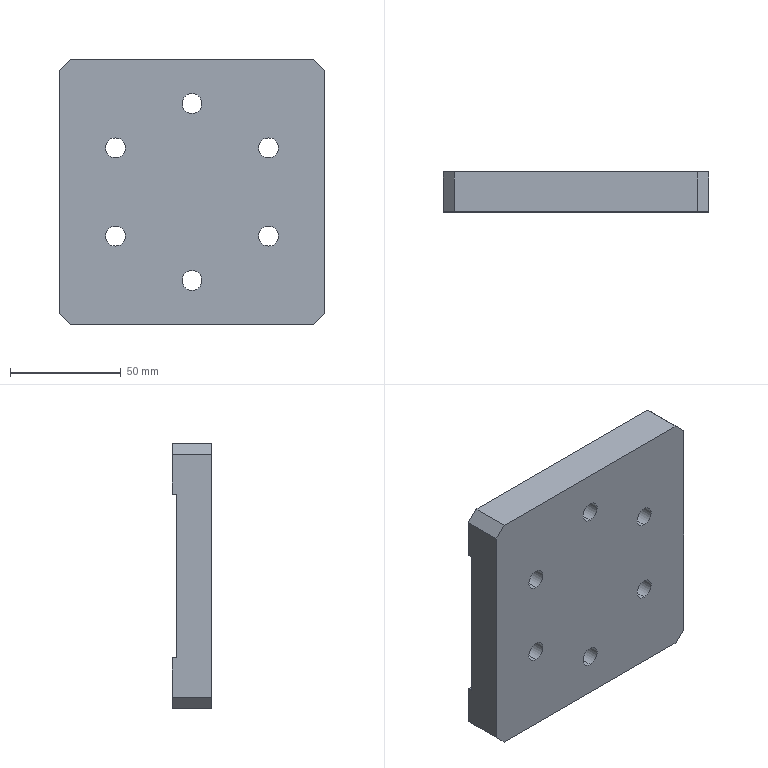Part | 1 solid | 46 faces | box 120 x 18 x 120 mm | volume 228068 mm3 | cylinder 24 | plane 22 | commonest cylinder face diameters 9 x12 15 x12
STEP:
#1=CARTESIAN_POINT('',(0.,7.4,-47.5));
#2=VERTEX_POINT('',#1);
#3=CARTESIAN_POINT('',(0.,7.4,-32.5));
#4=VERTEX_POINT('',#3);
#5=CARTESIAN_POINT('',(0.,7.4,-40.));
#6=DIRECTION('',(0.,1.,0.));
#7=DIRECTION('',(0.,0.,1.));
#8=AXIS2_PLACEMENT_3D('',#5,#6,#7);
#9=CIRCLE('',#8,7.5);
#10=EDGE_CURVE('',#2,#4,#9,.T.);
#11=ORIENTED_EDGE('',*,*,#10,.F.);
#12=CARTESIAN_POINT('',(0.,18.,-47.5));
#13=VERTEX_POINT('',#12);
#14=CARTESIAN_POINT('',(0.,18.,-47.5));
#15=DIRECTION('',(0.,1.,0.));
#16=VECTOR('',#15,1000.);
#17=LINE('',#14,#16);
#18=EDGE_CURVE('',#2,#13,#17,.T.);
#19=ORIENTED_EDGE('',*,*,#18,.T.);
#20=CARTESIAN_POINT('',(-6.874,18.,-37.));
#21=VERTEX_POINT('',#20);
#22=CARTESIAN_POINT('',(0.,18.,-40.));
#23=DIRECTION('',(0.,1.,0.));
#24=DIRECTION('',(0.,0.,1.));
#25=AXIS2_PLACEMENT_3D('',#22,#23,#24);
#26=CIRCLE('',#25,7.5);
#27=EDGE_CURVE('',#13,#21,#26,.T.);
#28=ORIENTED_EDGE('',*,*,#27,.T.);
#29=CARTESIAN_POINT('',(-6.874,16.,-37.));
#30=VERTEX_POINT('',#29);
#31=CARTESIAN_POINT('',(-6.874,18.,-37.));
#32=DIRECTION('',(0.,-1.,0.));
#33=VECTOR('',#32,1000.);
#34=LINE('',#31,#33);
#35=EDGE_CURVE('',#21,#30,#34,.T.);
#36=ORIENTED_EDGE('',*,*,#35,.T.);
#37=CARTESIAN_POINT('',(0.,16.,-32.5));
#38=VERTEX_POINT('',#37);
#39=CARTESIAN_POINT('',(0.,16.,-40.));
#40=DIRECTION('',(0.,1.,0.));
#41=DIRECTION('',(0.,0.,-1.));
#42=AXIS2_PLACEMENT_3D('',#39,#40,#41);
#43=CIRCLE('',#42,7.5);
#44=EDGE_CURVE('',#30,#38,#43,.T.);
#45=ORIENTED_EDGE('',*,*,#44,.T.);
#46=CARTESIAN_POINT('',(0.,18.,-32.5));
#47=DIRECTION('',(0.,1.,0.));
#48=VECTOR('',#47,1000.);
#49=LINE('',#46,#48);
#50=EDGE_CURVE('',#4,#38,#49,.T.);
#51=ORIENTED_EDGE('',*,*,#50,.F.);
#52=EDGE_LOOP('',(#11,#19,#28,#36,#45,#51));
#53=FACE_OUTER_BOUND('',#52,.T.);
#54=CARTESIAN_POINT('',(0.,18.,-40.));
#55=DIRECTION('',(0.,1.,0.));
#56=DIRECTION('',(0.,0.,1.));
#57=AXIS2_PLACEMENT_3D('',#54,#55,#56);
#58=CYLINDRICAL_SURFACE('',#57,7.5);
#59=ADVANCED_FACE('',(#53),#58,.F.);
#60=CARTESIAN_POINT('',(0.,0.,-44.5));
#61=VERTEX_POINT('',#60);
#62=CARTESIAN_POINT('',(0.,0.,-35.5));
#63=VERTEX_POINT('',#62);
#64=CARTESIAN_POINT('',(0.,0.,-40.));
#65=DIRECTION('',(0.,1.,0.));
#66=DIRECTION('',(0.,0.,1.));
#67=AXIS2_PLACEMENT_3D('',#64,#65,#66);
#68=CIRCLE('',#67,4.5);
#69=EDGE_CURVE('',#61,#63,#68,.T.);
#70=ORIENTED_EDGE('',*,*,#69,.F.);
#71=CARTESIAN_POINT('',(0.,7.4,-44.5));
#72=VERTEX_POINT('',#71);
#73=CARTESIAN_POINT('',(0.,18.,-44.5));
#74=DIRECTION('',(0.,1.,0.));
#75=VECTOR('',#74,1000.);
#76=LINE('',#73,#75);
#77=EDGE_CURVE('',#61,#72,#76,.T.);
#78=ORIENTED_EDGE('',*,*,#77,.T.);
#79=CARTESIAN_POINT('',(0.,7.4,-35.5));
#80=VERTEX_POINT('',#79);
#81=CARTESIAN_POINT('',(0.,7.4,-40.));
#82=DIRECTION('',(0.,1.,0.));
#83=DIRECTION('',(0.,0.,1.));
#84=AXIS2_PLACEMENT_3D('',#81,#82,#83);
#85=CIRCLE('',#84,4.5);
#86=EDGE_CURVE('',#72,#80,#85,.T.);
#87=ORIENTED_EDGE('',*,*,#86,.T.);
#88=CARTESIAN_POINT('',(0.,18.,-35.5));
#89=DIRECTION('',(0.,1.,0.));
#90=VECTOR('',#89,1000.);
#91=LINE('',#88,#90);
#92=EDGE_CURVE('',#63,#80,#91,.T.);
#93=ORIENTED_EDGE('',*,*,#92,.F.);
#94=EDGE_LOOP('',(#70,#78,#87,#93));
#95=FACE_OUTER_BOUND('',#94,.T.);
#96=CARTESIAN_POINT('',(0.,18.,-40.));
#97=DIRECTION('',(0.,1.,0.));
#98=DIRECTION('',(0.,0.,1.));
#99=AXIS2_PLACEMENT_3D('',#96,#97,#98);
#100=CYLINDRICAL_SURFACE('',#99,4.5);
#101=ADVANCED_FACE('',(#95),#100,.F.);
#102=CARTESIAN_POINT('',(-34.641,7.4,-27.5));
#103=VERTEX_POINT('',#102);
#104=CARTESIAN_POINT('',(-34.641,7.4,-12.5));
#105=VERTEX_POINT('',#104);
#106=CARTESIAN_POINT('',(-34.641,7.4,-20.));
#107=DIRECTION('',(0.,1.,0.));
#108=DIRECTION('',(0.,0.,1.));
#109=AXIS2_PLACEMENT_3D('',#106,#107,#108);
#110=CIRCLE('',#109,7.5);
#111=EDGE_CURVE('',#103,#105,#110,.T.);
#112=ORIENTED_EDGE('',*,*,#111,.F.);
#113=CARTESIAN_POINT('',(-34.641,16.,-27.5));
#114=VERTEX_POINT('',#113);
#115=CARTESIAN_POINT('',(-34.641,18.,-27.5));
#116=DIRECTION('',(0.,1.,0.));
#117=VECTOR('',#116,1000.);
#118=LINE('',#115,#117);
#119=EDGE_CURVE('',#103,#114,#118,.T.);
#120=ORIENTED_EDGE('',*,*,#119,.T.);
#121=CARTESIAN_POINT('',(-34.641,16.,-12.5));
#122=VERTEX_POINT('',#121);
#123=CARTESIAN_POINT('',(-34.641,16.,-20.));
#124=DIRECTION('',(0.,1.,0.));
#125=DIRECTION('',(0.,0.,-1.));
#126=AXIS2_PLACEMENT_3D('',#123,#124,#125);
#127=CIRCLE('',#126,7.5);
#128=EDGE_CURVE('',#114,#122,#127,.T.);
#129=ORIENTED_EDGE('',*,*,#128,.T.);
#130=CARTESIAN_POINT('',(-34.641,18.,-12.5));
#131=DIRECTION('',(0.,1.,0.));
#132=VECTOR('',#131,1000.);
#133=LINE('',#130,#132);
#134=EDGE_CURVE('',#105,#122,#133,.T.);
#135=ORIENTED_EDGE('',*,*,#134,.F.);
#136=EDGE_LOOP('',(#112,#120,#129,#135));
#137=FACE_OUTER_BOUND('',#136,.T.);
#138=CARTESIAN_POINT('',(-34.641,18.,-20.));
#139=DIRECTION('',(0.,1.,0.));
#140=DIRECTION('',(0.,0.,1.));
#141=AXIS2_PLACEMENT_3D('',#138,#139,#140);
#142=CYLINDRICAL_SURFACE('',#141,7.5);
#143=ADVANCED_FACE('',(#137),#142,.F.);
#144=CARTESIAN_POINT('',(-34.641,0.,-24.5));
#145=VERTEX_POINT('',#144);
#146=CARTESIAN_POINT('',(-34.641,0.,-15.5));
#147=VERTEX_POINT('',#146);
#148=CARTESIAN_POINT('',(-34.641,0.,-20.));
#149=DIRECTION('',(0.,1.,0.));
#150=DIRECTION('',(0.,0.,1.));
#151=AXIS2_PLACEMENT_3D('',#148,#149,#150);
#152=CIRCLE('',#151,4.5);
#153=EDGE_CURVE('',#145,#147,#152,.T.);
#154=ORIENTED_EDGE('',*,*,#153,.F.);
#155=CARTESIAN_POINT('',(-34.641,7.4,-24.5));
#156=VERTEX_POINT('',#155);
#157=CARTESIAN_POINT('',(-34.641,18.,-24.5));
#158=DIRECTION('',(0.,1.,0.));
#159=VECTOR('',#158,1000.);
#160=LINE('',#157,#159);
#161=EDGE_CURVE('',#145,#156,#160,.T.);
#162=ORIENTED_EDGE('',*,*,#161,.T.);
#163=CARTESIAN_POINT('',(-34.641,7.4,-15.5));
#164=VERTEX_POINT('',#163);
#165=CARTESIAN_POINT('',(-34.641,7.4,-20.));
#166=DIRECTION('',(0.,1.,0.));
#167=DIRECTION('',(0.,0.,1.));
#168=AXIS2_PLACEMENT_3D('',#165,#166,#167);
#169=CIRCLE('',#168,4.5);
#170=EDGE_CURVE('',#156,#164,#169,.T.);
#171=ORIENTED_EDGE('',*,*,#170,.T.);
#172=CARTESIAN_POINT('',(-34.641,18.,-15.5));
#173=DIRECTION('',(0.,1.,0.));
#174=VECTOR('',#173,1000.);
#175=LINE('',#172,#174);
#176=EDGE_CURVE('',#147,#164,#175,.T.);
#177=ORIENTED_EDGE('',*,*,#176,.F.);
#178=EDGE_LOOP('',(#154,#162,#171,#177));
#179=FACE_OUTER_BOUND('',#178,.T.);
#180=CARTESIAN_POINT('',(-34.641,18.,-20.));
#181=DIRECTION('',(0.,1.,0.));
#182=DIRECTION('',(0.,0.,1.));
#183=AXIS2_PLACEMENT_3D('',#180,#181,#182);
#184=CYLINDRICAL_SURFACE('',#183,4.5);
#185=ADVANCED_FACE('',(#179),#184,.F.);
#186=CARTESIAN_POINT('',(-34.641,7.4,12.5));
#187=VERTEX_POINT('',#186);
#188=CARTESIAN_POINT('',(-34.641,7.4,27.5));
#189=VERTEX_POINT('',#188);
#190=CARTESIAN_POINT('',(-34.641,7.4,20.));
#191=DIRECTION('',(0.,1.,0.));
#192=DIRECTION('',(0.,0.,1.));
#193=AXIS2_PLACEMENT_3D('',#190,#191,#192);
#194=CIRCLE('',#193,7.5);
#195=EDGE_CURVE('',#187,#189,#194,.T.);
#196=ORIENTED_EDGE('',*,*,#195,.F.);
#197=CARTESIAN_POINT('',(-34.641,16.,12.5));
#198=VERTEX_POINT('',#197);
#199=CARTESIAN_POINT('',(-34.641,18.,12.5));
#200=DIRECTION('',(0.,1.,0.));
#201=VECTOR('',#200,1000.);
#202=LINE('',#199,#201);
#203=EDGE_CURVE('',#187,#198,#202,.T.);
#204=ORIENTED_EDGE('',*,*,#203,.T.);
#205=CARTESIAN_POINT('',(-34.641,16.,27.5));
#206=VERTEX_POINT('',#205);
#207=CARTESIAN_POINT('',(-34.641,16.,20.));
#208=DIRECTION('',(0.,1.,0.));
#209=DIRECTION('',(0.,0.,-1.));
#210=AXIS2_PLACEMENT_3D('',#207,#208,#209);
#211=CIRCLE('',#210,7.5);
#212=EDGE_CURVE('',#198,#206,#211,.T.);
#213=ORIENTED_EDGE('',*,*,#212,.T.);
#214=CARTESIAN_POINT('',(-34.641,18.,27.5));
#215=DIRECTION('',(0.,1.,0.));
#216=VECTOR('',#215,1000.);
#217=LINE('',#214,#216);
#218=EDGE_CURVE('',#189,#206,#217,.T.);
#219=ORIENTED_EDGE('',*,*,#218,.F.);
#220=EDGE_LOOP('',(#196,#204,#213,#219));
#221=FACE_OUTER_BOUND('',#220,.T.);
#222=CARTESIAN_POINT('',(-34.641,18.,20.));
#223=DIRECTION('',(0.,1.,0.));
#224=DIRECTION('',(0.,0.,1.));
#225=AXIS2_PLACEMENT_3D('',#222,#223,#224);
#226=CYLINDRICAL_SURFACE('',#225,7.5);
#227=ADVANCED_FACE('',(#221),#226,.F.);
#228=CARTESIAN_POINT('',(-34.641,0.,15.5));
#229=VERTEX_POINT('',#228);
#230=CARTESIAN_POINT('',(-34.641,0.,24.5));
#231=VERTEX_POINT('',#230);
#232=CARTESIAN_POINT('',(-34.641,0.,20.));
#233=DIRECTION('',(0.,1.,0.));
#234=DIRECTION('',(0.,0.,1.));
#235=AXIS2_PLACEMENT_3D('',#232,#233,#234);
#236=CIRCLE('',#235,4.5);
#237=EDGE_CURVE('',#229,#231,#236,.T.);
#238=ORIENTED_EDGE('',*,*,#237,.F.);
#239=CARTESIAN_POINT('',(-34.641,7.4,15.5));
#240=VERTEX_POINT('',#239);
#241=CARTESIAN_POINT('',(-34.641,18.,15.5));
#242=DIRECTION('',(0.,1.,0.));
#243=VECTOR('',#242,1000.);
#244=LINE('',#241,#243);
#245=EDGE_CURVE('',#229,#240,#244,.T.);
#246=ORIENTED_EDGE('',*,*,#245,.T.);
#247=CARTESIAN_POINT('',(-34.641,7.4,24.5));
#248=VERTEX_POINT('',#247);
#249=CARTESIAN_POINT('',(-34.641,7.4,20.));
#250=DIRECTION('',(0.,1.,0.));
#251=DIRECTION('',(0.,0.,1.));
#252=AXIS2_PLACEMENT_3D('',#249,#250,#251);
#253=CIRCLE('',#252,4.5);
#254=EDGE_CURVE('',#240,#248,#253,.T.);
#255=ORIENTED_EDGE('',*,*,#254,.T.);
#256=CARTESIAN_POINT('',(-34.641,18.,24.5));
#257=DIRECTION('',(0.,1.,0.));
#258=VECTOR('',#257,1000.);
#259=LINE('',#256,#258);
#260=EDGE_CURVE('',#231,#248,#259,.T.);
#261=ORIENTED_EDGE('',*,*,#260,.F.);
#262=EDGE_LOOP('',(#238,#246,#255,#261));
#263=FACE_OUTER_BOUND('',#262,.T.);
#264=CARTESIAN_POINT('',(-34.641,18.,20.));
#265=DIRECTION('',(0.,1.,0.));
#266=DIRECTION('',(0.,0.,1.));
#267=AXIS2_PLACEMENT_3D('',#264,#265,#266);
#268=CYLINDRICAL_SURFACE('',#267,4.5);
#269=ADVANCED_FACE('',(#263),#268,.F.);
#270=CARTESIAN_POINT('',(0.,7.4,32.5));
#271=VERTEX_POINT('',#270);
#272=CARTESIAN_POINT('',(0.,7.4,47.5));
#273=VERTEX_POINT('',#272);
#274=CARTESIAN_POINT('',(0.,7.4,40.));
#275=DIRECTION('',(0.,1.,0.));
#276=DIRECTION('',(0.,0.,1.));
#277=AXIS2_PLACEMENT_3D('',#274,#275,#276);
#278=CIRCLE('',#277,7.5);
#279=EDGE_CURVE('',#271,#273,#278,.T.);
#280=ORIENTED_EDGE('',*,*,#279,.F.);
#281=CARTESIAN_POINT('',(0.,16.,32.5));
#282=VERTEX_POINT('',#281);
#283=CARTESIAN_POINT('',(0.,18.,32.5));
#284=DIRECTION('',(0.,1.,0.));
#285=VECTOR('',#284,1000.);
#286=LINE('',#283,#285);
#287=EDGE_CURVE('',#271,#282,#286,.T.);
#288=ORIENTED_EDGE('',*,*,#287,.T.);
#289=CARTESIAN_POINT('',(-6.874,16.,37.));
#290=VERTEX_POINT('',#289);
#291=CARTESIAN_POINT('',(0.,16.,40.));
#292=DIRECTION('',(0.,1.,0.));
#293=DIRECTION('',(0.,0.,-1.));
#294=AXIS2_PLACEMENT_3D('',#291,#292,#293);
#295=CIRCLE('',#294,7.5);
#296=EDGE_CURVE('',#282,#290,#295,.T.);
#297=ORIENTED_EDGE('',*,*,#296,.T.);
#298=CARTESIAN_POINT('',(-6.874,18.,37.));
#299=VERTEX_POINT('',#298);
#300=CARTESIAN_POINT('',(-6.874,18.,37.));
#301=DIRECTION('',(0.,1.,0.));
#302=VECTOR('',#301,1000.);
#303=LINE('',#300,#302);
#304=EDGE_CURVE('',#290,#299,#303,.T.);
#305=ORIENTED_EDGE('',*,*,#304,.T.);
#306=CARTESIAN_POINT('',(0.,18.,47.5));
#307=VERTEX_POINT('',#306);
#308=CARTESIAN_POINT('',(0.,18.,40.));
#309=DIRECTION('',(0.,1.,0.));
#310=DIRECTION('',(0.,0.,1.));
#311=AXIS2_PLACEMENT_3D('',#308,#309,#310);
#312=CIRCLE('',#311,7.5);
#313=EDGE_CURVE('',#299,#307,#312,.T.);
#314=ORIENTED_EDGE('',*,*,#313,.T.);
#315=CARTESIAN_POINT('',(0.,18.,47.5));
#316=DIRECTION('',(0.,1.,0.));
#317=VECTOR('',#316,1000.);
#318=LINE('',#315,#317);
#319=EDGE_CURVE('',#273,#307,#318,.T.);
#320=ORIENTED_EDGE('',*,*,#319,.F.);
#321=EDGE_LOOP('',(#280,#288,#297,#305,#314,#320));
#322=FACE_OUTER_BOUND('',#321,.T.);
#323=CARTESIAN_POINT('',(0.,18.,40.));
#324=DIRECTION('',(0.,1.,0.));
#325=DIRECTION('',(0.,0.,1.));
#326=AXIS2_PLACEMENT_3D('',#323,#324,#325);
#327=CYLINDRICAL_SURFACE('',#326,7.5);
#328=ADVANCED_FACE('',(#322),#327,.F.);
#329=CARTESIAN_POINT('',(0.,0.,35.5));
#330=VERTEX_POINT('',#329);
#331=CARTESIAN_POINT('',(0.,0.,44.5));
#332=VERTEX_POINT('',#331);
#333=CARTESIAN_POINT('',(0.,0.,40.));
#334=DIRECTION('',(0.,1.,0.));
#335=DIRECTION('',(0.,0.,1.));
#336=AXIS2_PLACEMENT_3D('',#333,#334,#335);
#337=CIRCLE('',#336,4.5);
#338=EDGE_CURVE('',#330,#332,#337,.T.);
#339=ORIENTED_EDGE('',*,*,#338,.F.);
#340=CARTESIAN_POINT('',(0.,7.4,35.5));
#341=VERTEX_POINT('',#340);
#342=CARTESIAN_POINT('',(0.,18.,35.5));
#343=DIRECTION('',(0.,1.,0.));
#344=VECTOR('',#343,1000.);
#345=LINE('',#342,#344);
#346=EDGE_CURVE('',#330,#341,#345,.T.);
#347=ORIENTED_EDGE('',*,*,#346,.T.);
#348=CARTESIAN_POINT('',(0.,7.4,44.5));
#349=VERTEX_POINT('',#348);
#350=CARTESIAN_POINT('',(0.,7.4,40.));
#351=DIRECTION('',(0.,1.,0.));
#352=DIRECTION('',(0.,0.,1.));
#353=AXIS2_PLACEMENT_3D('',#350,#351,#352);
#354=CIRCLE('',#353,4.5);
#355=EDGE_CURVE('',#341,#349,#354,.T.);
#356=ORIENTED_EDGE('',*,*,#355,.T.);
#357=CARTESIAN_POINT('',(0.,18.,44.5));
#358=DIRECTION('',(0.,1.,0.));
#359=VECTOR('',#358,1000.);
#360=LINE('',#357,#359);
#361=EDGE_CURVE('',#332,#349,#360,.T.);
#362=ORIENTED_EDGE('',*,*,#361,.F.);
#363=EDGE_LOOP('',(#339,#347,#356,#362));
#364=FACE_OUTER_BOUND('',#363,.T.);
#365=CARTESIAN_POINT('',(0.,18.,40.));
#366=DIRECTION('',(0.,1.,0.));
#367=DIRECTION('',(0.,0.,1.));
#368=AXIS2_PLACEMENT_3D('',#365,#366,#367);
#369=CYLINDRICAL_SURFACE('',#368,4.5);
#370=ADVANCED_FACE('',(#364),#369,.F.);
#371=CARTESIAN_POINT('',(34.641,7.4,12.5));
#372=VERTEX_POINT('',#371);
#373=CARTESIAN_POINT('',(34.641,7.4,27.5));
#374=VERTEX_POINT('',#373);
#375=CARTESIAN_POINT('',(34.641,7.4,20.));
#376=DIRECTION('',(0.,1.,0.));
#377=DIRECTION('',(0.,0.,1.));
#378=AXIS2_PLACEMENT_3D('',#375,#376,#377);
#379=CIRCLE('',#378,7.5);
#380=EDGE_CURVE('',#372,#374,#379,.T.);
#381=ORIENTED_EDGE('',*,*,#380,.F.);
#382=CARTESIAN_POINT('',(34.641,16.,12.5));
#383=VERTEX_POINT('',#382);
#384=CARTESIAN_POINT('',(34.641,18.,12.5));
#385=DIRECTION('',(0.,1.,0.));
#386=VECTOR('',#385,1000.);
#387=LINE('',#384,#386);
#388=EDGE_CURVE('',#372,#383,#387,.T.);
#389=ORIENTED_EDGE('',*,*,#388,.T.);
#390=CARTESIAN_POINT('',(34.641,16.,27.5));
#391=VERTEX_POINT('',#390);
#392=CARTESIAN_POINT('',(34.641,16.,20.));
#393=DIRECTION('',(0.,1.,0.));
#394=DIRECTION('',(0.,0.,-1.));
#395=AXIS2_PLACEMENT_3D('',#392,#393,#394);
#396=CIRCLE('',#395,7.5);
#397=EDGE_CURVE('',#383,#391,#396,.T.);
#398=ORIENTED_EDGE('',*,*,#397,.T.);
#399=CARTESIAN_POINT('',(34.641,18.,27.5));
#400=DIRECTION('',(0.,1.,0.));
#401=VECTOR('',#400,1000.);
#402=LINE('',#399,#401);
#403=EDGE_CURVE('',#374,#391,#402,.T.);
#404=ORIENTED_EDGE('',*,*,#403,.F.);
#405=EDGE_LOOP('',(#381,#389,#398,#404));
#406=FACE_OUTER_BOUND('',#405,.T.);
#407=CARTESIAN_POINT('',(34.641,18.,20.));
#408=DIRECTION('',(0.,1.,0.));
#409=DIRECTION('',(0.,0.,1.));
#410=AXIS2_PLACEMENT_3D('',#407,#408,#409);
#411=CYLINDRICAL_SURFACE('',#410,7.5);
#412=ADVANCED_FACE('',(#406),#411,.F.);
#413=CARTESIAN_POINT('',(34.641,0.,15.5));
#414=VERTEX_POINT('',#413);
#415=CARTESIAN_POINT('',(34.641,0.,24.5));
#416=VERTEX_POINT('',#415);
#417=CARTESIAN_POINT('',(34.641,0.,20.));
#418=DIRECTION('',(0.,1.,0.));
#419=DIRECTION('',(0.,0.,1.));
#420=AXIS2_PLACEMENT_3D('',#417,#418,#419);
#421=CIRCLE('',#420,4.5);
#422=EDGE_CURVE('',#414,#416,#421,.T.);
#423=ORIENTED_EDGE('',*,*,#422,.F.);
#424=CARTESIAN_POINT('',(34.641,7.4,15.5));
#425=VERTEX_POINT('',#424);
#426=CARTESIAN_POINT('',(34.641,18.,15.5));
#427=DIRECTION('',(0.,1.,0.));
#428=VECTOR('',#427,1000.);
#429=LINE('',#426,#428);
#430=EDGE_CURVE('',#414,#425,#429,.T.);
#431=ORIENTED_EDGE('',*,*,#430,.T.);
#432=CARTESIAN_POINT('',(34.641,7.4,24.5));
#433=VERTEX_POINT('',#432);
#434=CARTESIAN_POINT('',(34.641,7.4,20.));
#435=DIRECTION('',(0.,1.,0.));
#436=DIRECTION('',(0.,0.,1.));
#437=AXIS2_PLACEMENT_3D('',#434,#435,#436);
#438=CIRCLE('',#437,4.5);
#439=EDGE_CURVE('',#425,#433,#438,.T.);
#440=ORIENTED_EDGE('',*,*,#439,.T.);
#441=CARTESIAN_POINT('',(34.641,18.,24.5));
#442=DIRECTION('',(0.,1.,0.));
#443=VECTOR('',#442,1000.);
#444=LINE('',#441,#443);
#445=EDGE_CURVE('',#416,#433,#444,.T.);
#446=ORIENTED_EDGE('',*,*,#445,.F.);
#447=EDGE_LOOP('',(#423,#431,#440,#446));
#448=FACE_OUTER_BOUND('',#447,.T.);
#449=CARTESIAN_POINT('',(34.641,18.,20.));
#450=DIRECTION('',(0.,1.,0.));
#451=DIRECTION('',(0.,0.,1.));
#452=AXIS2_PLACEMENT_3D('',#449,#450,#451);
#453=CYLINDRICAL_SURFACE('',#452,4.5);
#454=ADVANCED_FACE('',(#448),#453,.F.);
#455=CARTESIAN_POINT('',(34.641,7.4,-27.5));
#456=VERTEX_POINT('',#455);
#457=CARTESIAN_POINT('',(34.641,7.4,-12.5));
#458=VERTEX_POINT('',#457);
#459=CARTESIAN_POINT('',(34.641,7.4,-20.));
#460=DIRECTION('',(0.,1.,0.));
#461=DIRECTION('',(0.,0.,1.));
#462=AXIS2_PLACEMENT_3D('',#459,#460,#461);
#463=CIRCLE('',#462,7.5);
#464=EDGE_CURVE('',#456,#458,#463,.T.);
#465=ORIENTED_EDGE('',*,*,#464,.F.);
#466=CARTESIAN_POINT('',(34.641,16.,-27.5));
#467=VERTEX_POINT('',#466);
#468=CARTESIAN_POINT('',(34.641,18.,-27.5));
#469=DIRECTION('',(0.,1.,0.));
#470=VECTOR('',#469,1000.);
#471=LINE('',#468,#470);
#472=EDGE_CURVE('',#456,#467,#471,.T.);
#473=ORIENTED_EDGE('',*,*,#472,.T.);
#474=CARTESIAN_POINT('',(34.641,16.,-12.5));
#475=VERTEX_POINT('',#474);
#476=CARTESIAN_POINT('',(34.641,16.,-20.));
#477=DIRECTION('',(0.,1.,0.));
#478=DIRECTION('',(0.,0.,-1.));
#479=AXIS2_PLACEMENT_3D('',#476,#477,#478);
#480=CIRCLE('',#479,7.5);
#481=EDGE_CURVE('',#467,#475,#480,.T.);
#482=ORIENTED_EDGE('',*,*,#481,.T.);
#483=CARTESIAN_POINT('',(34.641,18.,-12.5));
#484=DIRECTION('',(0.,1.,0.));
#485=VECTOR('',#484,1000.);
#486=LINE('',#483,#485);
#487=EDGE_CURVE('',#458,#475,#486,.T.);
#488=ORIENTED_EDGE('',*,*,#487,.F.);
#489=EDGE_LOOP('',(#465,#473,#482,#488));
#490=FACE_OUTER_BOUND('',#489,.T.);
#491=CARTESIAN_POINT('',(34.641,18.,-20.));
#492=DIRECTION('',(0.,1.,0.));
#493=DIRECTION('',(0.,0.,1.));
#494=AXIS2_PLACEMENT_3D('',#491,#492,#493);
#495=CYLINDRICAL_SURFACE('',#494,7.5);
#496=ADVANCED_FACE('',(#490),#495,.F.);
#497=CARTESIAN_POINT('',(34.641,0.,-24.5));
#498=VERTEX_POINT('',#497);
#499=CARTESIAN_POINT('',(34.641,0.,-15.5));
#500=VERTEX_POINT('',#499);
#501=CARTESIAN_POINT('',(34.641,0.,-20.));
#502=DIRECTION('',(0.,1.,0.));
#503=DIRECTION('',(0.,0.,1.));
#504=AXIS2_PLACEMENT_3D('',#501,#502,#503);
#505=CIRCLE('',#504,4.5);
#506=EDGE_CURVE('',#498,#500,#505,.T.);
#507=ORIENTED_EDGE('',*,*,#506,.F.);
#508=CARTESIAN_POINT('',(34.641,7.4,-24.5));
#509=VERTEX_POINT('',#508);
#510=CARTESIAN_POINT('',(34.641,18.,-24.5));
#511=DIRECTION('',(0.,1.,0.));
#512=VECTOR('',#511,1000.);
#513=LINE('',#510,#512);
#514=EDGE_CURVE('',#498,#509,#513,.T.);
#515=ORIENTED_EDGE('',*,*,#514,.T.);
#516=CARTESIAN_POINT('',(34.641,7.4,-15.5));
#517=VERTEX_POINT('',#516);
#518=CARTESIAN_POINT('',(34.641,7.4,-20.));
#519=DIRECTION('',(0.,1.,0.));
#520=DIRECTION('',(0.,0.,1.));
#521=AXIS2_PLACEMENT_3D('',#518,#519,#520);
#522=CIRCLE('',#521,4.5);
#523=EDGE_CURVE('',#509,#517,#522,.T.);
#524=ORIENTED_EDGE('',*,*,#523,.T.);
#525=CARTESIAN_POINT('',(34.641,18.,-15.5));
#526=DIRECTION('',(0.,1.,0.));
#527=VECTOR('',#526,1000.);
#528=LINE('',#525,#527);
#529=EDGE_CURVE('',#500,#517,#528,.T.);
#530=ORIENTED_EDGE('',*,*,#529,.F.);
#531=EDGE_LOOP('',(#507,#515,#524,#530));
#532=FACE_OUTER_BOUND('',#531,.T.);
#533=CARTESIAN_POINT('',(34.641,18.,-20.));
#534=DIRECTION('',(0.,1.,0.));
#535=DIRECTION('',(0.,0.,1.));
#536=AXIS2_PLACEMENT_3D('',#533,#534,#535);
#537=CYLINDRICAL_SURFACE('',#536,4.5);
#538=ADVANCED_FACE('',(#532),#537,.F.);
#539=CARTESIAN_POINT('',(-55.,18.,60.));
#540=VERTEX_POINT('',#539);
#541=CARTESIAN_POINT('',(55.,18.,60.));
#542=VERTEX_POINT('',#541);
#543=CARTESIAN_POINT('',(-60.,18.,60.));
#544=DIRECTION('',(1.,0.,0.));
#545=VECTOR('',#544,1000.);
#546=LINE('',#543,#545);
#547=EDGE_CURVE('',#540,#542,#546,.T.);
#548=ORIENTED_EDGE('',*,*,#547,.T.);
#549=CARTESIAN_POINT('',(60.,18.,55.));
#550=VERTEX_POINT('',#549);
#551=CARTESIAN_POINT('',(60.,18.,55.));
#552=DIRECTION('',(0.7071,0.,-0.7071));
#553=VECTOR('',#552,1000.);
#554=LINE('',#551,#553);
#555=EDGE_CURVE('',#542,#550,#554,.T.);
#556=ORIENTED_EDGE('',*,*,#555,.T.);
#557=CARTESIAN_POINT('',(60.,18.,37.));
#558=VERTEX_POINT('',#557);
#559=CARTESIAN_POINT('',(60.,18.,60.));
#560=DIRECTION('',(0.,0.,-1.));
#561=VECTOR('',#560,1000.);
#562=LINE('',#559,#561);
#563=EDGE_CURVE('',#550,#558,#562,.T.);
#564=ORIENTED_EDGE('',*,*,#563,.T.);
#565=CARTESIAN_POINT('',(6.874,18.,37.));
#566=VERTEX_POINT('',#565);
#567=CARTESIAN_POINT('',(-60.,18.,37.));
#568=DIRECTION('',(1.,0.,0.));
#569=VECTOR('',#568,1000.);
#570=LINE('',#567,#569);
#571=EDGE_CURVE('',#566,#558,#570,.T.);
#572=ORIENTED_EDGE('',*,*,#571,.F.);
#573=CARTESIAN_POINT('',(0.,18.,40.));
#574=DIRECTION('',(0.,1.,0.));
#575=DIRECTION('',(0.,0.,1.));
#576=AXIS2_PLACEMENT_3D('',#573,#574,#575);
#577=CIRCLE('',#576,7.5);
#578=EDGE_CURVE('',#307,#566,#577,.T.);
#579=ORIENTED_EDGE('',*,*,#578,.F.);
#580=ORIENTED_EDGE('',*,*,#313,.F.);
#581=CARTESIAN_POINT('',(-60.,18.,37.));
#582=VERTEX_POINT('',#581);
#583=CARTESIAN_POINT('',(-60.,18.,37.));
#584=DIRECTION('',(1.,0.,0.));
#585=VECTOR('',#584,1000.);
#586=LINE('',#583,#585);
#587=EDGE_CURVE('',#582,#299,#586,.T.);
#588=ORIENTED_EDGE('',*,*,#587,.F.);
#589=CARTESIAN_POINT('',(-60.,18.,55.));
#590=VERTEX_POINT('',#589);
#591=CARTESIAN_POINT('',(-60.,18.,60.));
#592=DIRECTION('',(0.,0.,1.));
#593=VECTOR('',#592,1000.);
#594=LINE('',#591,#593);
#595=EDGE_CURVE('',#582,#590,#594,.T.);
#596=ORIENTED_EDGE('',*,*,#595,.T.);
#597=CARTESIAN_POINT('',(-55.,18.,60.));
#598=DIRECTION('',(0.7071,0.,0.7071));
#599=VECTOR('',#598,1000.);
#600=LINE('',#597,#599);
#601=EDGE_CURVE('',#590,#540,#600,.T.);
#602=ORIENTED_EDGE('',*,*,#601,.T.);
#603=EDGE_LOOP('',(#548,#556,#564,#572,#579,#580,#588,#596,#602));
#604=FACE_OUTER_BOUND('',#603,.T.);
#605=CARTESIAN_POINT('',(0.,18.,0.));
#606=DIRECTION('',(0.,-1.,0.));
#607=DIRECTION('',(0.,0.,-1.));
#608=AXIS2_PLACEMENT_3D('',#605,#606,#607);
#609=PLANE('',#608);
#610=ADVANCED_FACE('',(#604),#609,.F.);
#611=ORIENTED_EDGE('',*,*,#563,.F.);
#612=CARTESIAN_POINT('',(60.,0.,55.));
#613=VERTEX_POINT('',#612);
#614=CARTESIAN_POINT('',(60.,18.,55.));
#615=DIRECTION('',(0.,-1.,0.));
#616=VECTOR('',#615,1000.);
#617=LINE('',#614,#616);
#618=EDGE_CURVE('',#550,#613,#617,.T.);
#619=ORIENTED_EDGE('',*,*,#618,.T.);
#620=CARTESIAN_POINT('',(60.,0.,-55.));
#621=VERTEX_POINT('',#620);
#622=CARTESIAN_POINT('',(60.,0.,60.));
#623=DIRECTION('',(0.,0.,-1.));
#624=VECTOR('',#623,1000.);
#625=LINE('',#622,#624);
#626=EDGE_CURVE('',#613,#621,#625,.T.);
#627=ORIENTED_EDGE('',*,*,#626,.T.);
#628=CARTESIAN_POINT('',(60.,18.,-55.));
#629=VERTEX_POINT('',#628);
#630=CARTESIAN_POINT('',(60.,18.,-55.));
#631=DIRECTION('',(0.,1.,0.));
#632=VECTOR('',#631,1000.);
#633=LINE('',#630,#632);
#634=EDGE_CURVE('',#621,#629,#633,.T.);
#635=ORIENTED_EDGE('',*,*,#634,.T.);
#636=CARTESIAN_POINT('',(60.,18.,-37.));
#637=VERTEX_POINT('',#636);
#638=CARTESIAN_POINT('',(60.,18.,60.));
#639=DIRECTION('',(0.,0.,-1.));
#640=VECTOR('',#639,1000.);
#641=LINE('',#638,#640);
#642=EDGE_CURVE('',#637,#629,#641,.T.);
#643=ORIENTED_EDGE('',*,*,#642,.F.);
#644=CARTESIAN_POINT('',(60.,16.,-37.));
#645=VERTEX_POINT('',#644);
#646=CARTESIAN_POINT('',(60.,16.,-37.));
#647=DIRECTION('',(0.,1.,0.));
#648=VECTOR('',#647,1000.);
#649=LINE('',#646,#648);
#650=EDGE_CURVE('',#645,#637,#649,.T.);
#651=ORIENTED_EDGE('',*,*,#650,.F.);
#652=CARTESIAN_POINT('',(60.,16.,37.));
#653=VERTEX_POINT('',#652);
#654=CARTESIAN_POINT('',(60.,16.,37.));
#655=DIRECTION('',(0.,0.,-1.));
#656=VECTOR('',#655,1000.);
#657=LINE('',#654,#656);
#658=EDGE_CURVE('',#653,#645,#657,.T.);
#659=ORIENTED_EDGE('',*,*,#658,.F.);
#660=CARTESIAN_POINT('',(60.,16.,37.));
#661=DIRECTION('',(0.,1.,0.));
#662=VECTOR('',#661,1000.);
#663=LINE('',#660,#662);
#664=EDGE_CURVE('',#653,#558,#663,.T.);
#665=ORIENTED_EDGE('',*,*,#664,.T.);
#666=EDGE_LOOP('',(#611,#619,#627,#635,#643,#651,#659,#665));
#667=FACE_OUTER_BOUND('',#666,.T.);
#668=CARTESIAN_POINT('',(60.,18.,60.));
#669=DIRECTION('',(-1.,0.,0.));
#670=DIRECTION('',(0.,0.,1.));
#671=AXIS2_PLACEMENT_3D('',#668,#669,#670);
#672=PLANE('',#671);
#673=ADVANCED_FACE('',(#667),#672,.F.);
#674=CARTESIAN_POINT('',(55.,0.,-60.));
#675=VERTEX_POINT('',#674);
#676=CARTESIAN_POINT('',(-55.,0.,-60.));
#677=VERTEX_POINT('',#676);
#678=CARTESIAN_POINT('',(-60.,0.,-60.));
#679=DIRECTION('',(-1.,0.,0.));
#680=VECTOR('',#679,1000.);
#681=LINE('',#678,#680);
#682=EDGE_CURVE('',#675,#677,#681,.T.);
#683=ORIENTED_EDGE('',*,*,#682,.T.);
#684=CARTESIAN_POINT('',(-55.,18.,-60.));
#685=VERTEX_POINT('',#684);
#686=CARTESIAN_POINT('',(-55.,18.,-60.));
#687=DIRECTION('',(0.,1.,0.));
#688=VECTOR('',#687,1000.);
#689=LINE('',#686,#688);
#690=EDGE_CURVE('',#677,#685,#689,.T.);
#691=ORIENTED_EDGE('',*,*,#690,.T.);
#692=CARTESIAN_POINT('',(55.,18.,-60.));
#693=VERTEX_POINT('',#692);
#694=CARTESIAN_POINT('',(-60.,18.,-60.));
#695=DIRECTION('',(-1.,0.,0.));
#696=VECTOR('',#695,1000.);
#697=LINE('',#694,#696);
#698=EDGE_CURVE('',#693,#685,#697,.T.);
#699=ORIENTED_EDGE('',*,*,#698,.F.);
#700=CARTESIAN_POINT('',(55.,18.,-60.));
#701=DIRECTION('',(0.,-1.,0.));
#702=VECTOR('',#701,1000.);
#703=LINE('',#700,#702);
#704=EDGE_CURVE('',#693,#675,#703,.T.);
#705=ORIENTED_EDGE('',*,*,#704,.T.);
#706=EDGE_LOOP('',(#683,#691,#699,#705));
#707=FACE_OUTER_BOUND('',#706,.T.);
#708=CARTESIAN_POINT('',(-60.,18.,-60.));
#709=DIRECTION('',(0.,0.,1.));
#710=DIRECTION('',(1.,0.,0.));
#711=AXIS2_PLACEMENT_3D('',#708,#709,#710);
#712=PLANE('',#711);
#713=ADVANCED_FACE('',(#707),#712,.F.);
#714=CARTESIAN_POINT('',(-60.,0.,-55.));
#715=VERTEX_POINT('',#714);
#716=CARTESIAN_POINT('',(-60.,0.,55.));
#717=VERTEX_POINT('',#716);
#718=CARTESIAN_POINT('',(-60.,0.,60.));
#719=DIRECTION('',(0.,0.,1.));
#720=VECTOR('',#719,1000.);
#721=LINE('',#718,#720);
#722=EDGE_CURVE('',#715,#717,#721,.T.);
#723=ORIENTED_EDGE('',*,*,#722,.T.);
#724=CARTESIAN_POINT('',(-60.,18.,55.));
#725=DIRECTION('',(0.,1.,0.));
#726=VECTOR('',#725,1000.);
#727=LINE('',#724,#726);
#728=EDGE_CURVE('',#717,#590,#727,.T.);
#729=ORIENTED_EDGE('',*,*,#728,.T.);
#730=ORIENTED_EDGE('',*,*,#595,.F.);
#731=CARTESIAN_POINT('',(-60.,16.,37.));
#732=VERTEX_POINT('',#731);
#733=CARTESIAN_POINT('',(-60.,16.,37.));
#734=DIRECTION('',(0.,1.,0.));
#735=VECTOR('',#734,1000.);
#736=LINE('',#733,#735);
#737=EDGE_CURVE('',#732,#582,#736,.T.);
#738=ORIENTED_EDGE('',*,*,#737,.F.);
#739=CARTESIAN_POINT('',(-60.,16.,-37.));
#740=VERTEX_POINT('',#739);
#741=CARTESIAN_POINT('',(-60.,16.,37.));
#742=DIRECTION('',(0.,0.,1.));
#743=VECTOR('',#742,1000.);
#744=LINE('',#741,#743);
#745=EDGE_CURVE('',#740,#732,#744,.T.);
#746=ORIENTED_EDGE('',*,*,#745,.F.);
#747=CARTESIAN_POINT('',(-60.,18.,-37.));
#748=VERTEX_POINT('',#747);
#749=CARTESIAN_POINT('',(-60.,16.,-37.));
#750=DIRECTION('',(0.,1.,0.));
#751=VECTOR('',#750,1000.);
#752=LINE('',#749,#751);
#753=EDGE_CURVE('',#740,#748,#752,.T.);
#754=ORIENTED_EDGE('',*,*,#753,.T.);
#755=CARTESIAN_POINT('',(-60.,18.,-55.));
#756=VERTEX_POINT('',#755);
#757=CARTESIAN_POINT('',(-60.,18.,60.));
#758=DIRECTION('',(0.,0.,1.));
#759=VECTOR('',#758,1000.);
#760=LINE('',#757,#759);
#761=EDGE_CURVE('',#756,#748,#760,.T.);
#762=ORIENTED_EDGE('',*,*,#761,.F.);
#763=CARTESIAN_POINT('',(-60.,18.,-55.));
#764=DIRECTION('',(0.,-1.,0.));
#765=VECTOR('',#764,1000.);
#766=LINE('',#763,#765);
#767=EDGE_CURVE('',#756,#715,#766,.T.);
#768=ORIENTED_EDGE('',*,*,#767,.T.);
#769=EDGE_LOOP('',(#723,#729,#730,#738,#746,#754,#762,#768));
#770=FACE_OUTER_BOUND('',#769,.T.);
#771=CARTESIAN_POINT('',(-60.,18.,60.));
#772=DIRECTION('',(1.,0.,0.));
#773=DIRECTION('',(0.,0.,-1.));
#774=AXIS2_PLACEMENT_3D('',#771,#772,#773);
#775=PLANE('',#774);
#776=ADVANCED_FACE('',(#770),#775,.F.);
#777=CARTESIAN_POINT('',(-55.,0.,60.));
#778=VERTEX_POINT('',#777);
#779=CARTESIAN_POINT('',(55.,0.,60.));
#780=VERTEX_POINT('',#779);
#781=CARTESIAN_POINT('',(-60.,0.,60.));
#782=DIRECTION('',(1.,0.,0.));
#783=VECTOR('',#782,1000.);
#784=LINE('',#781,#783);
#785=EDGE_CURVE('',#778,#780,#784,.T.);
#786=ORIENTED_EDGE('',*,*,#785,.T.);
#787=CARTESIAN_POINT('',(55.,18.,60.));
#788=DIRECTION('',(0.,1.,0.));
#789=VECTOR('',#788,1000.);
#790=LINE('',#787,#789);
#791=EDGE_CURVE('',#780,#542,#790,.T.);
#792=ORIENTED_EDGE('',*,*,#791,.T.);
#793=ORIENTED_EDGE('',*,*,#547,.F.);
#794=CARTESIAN_POINT('',(-55.,18.,60.));
#795=DIRECTION('',(0.,-1.,0.));
#796=VECTOR('',#795,1000.);
#797=LINE('',#794,#796);
#798=EDGE_CURVE('',#540,#778,#797,.T.);
#799=ORIENTED_EDGE('',*,*,#798,.T.);
#800=EDGE_LOOP('',(#786,#792,#793,#799));
#801=FACE_OUTER_BOUND('',#800,.T.);
#802=CARTESIAN_POINT('',(-60.,18.,60.));
#803=DIRECTION('',(0.,0.,-1.));
#804=DIRECTION('',(-1.,0.,0.));
#805=AXIS2_PLACEMENT_3D('',#802,#803,#804);
#806=PLANE('',#805);
#807=ADVANCED_FACE('',(#801),#806,.F.);
#808=ORIENTED_EDGE('',*,*,#698,.T.);
#809=CARTESIAN_POINT('',(-60.,18.,-55.));
#810=DIRECTION('',(-0.7071,0.,0.7071));
#811=VECTOR('',#810,1000.);
#812=LINE('',#809,#811);
#813=EDGE_CURVE('',#685,#756,#812,.T.);
#814=ORIENTED_EDGE('',*,*,#813,.T.);
#815=ORIENTED_EDGE('',*,*,#761,.T.);
#816=CARTESIAN_POINT('',(-60.,18.,-37.));
#817=DIRECTION('',(-1.,0.,0.));
#818=VECTOR('',#817,1000.);
#819=LINE('',#816,#818);
#820=EDGE_CURVE('',#21,#748,#819,.T.);
#821=ORIENTED_EDGE('',*,*,#820,.F.);
#822=ORIENTED_EDGE('',*,*,#27,.F.);
#823=CARTESIAN_POINT('',(6.874,18.,-37.));
#824=VERTEX_POINT('',#823);
#825=CARTESIAN_POINT('',(0.,18.,-40.));
#826=DIRECTION('',(0.,1.,0.));
#827=DIRECTION('',(0.,0.,1.));
#828=AXIS2_PLACEMENT_3D('',#825,#826,#827);
#829=CIRCLE('',#828,7.5);
#830=EDGE_CURVE('',#824,#13,#829,.T.);
#831=ORIENTED_EDGE('',*,*,#830,.F.);
#832=CARTESIAN_POINT('',(-60.,18.,-37.));
#833=DIRECTION('',(-1.,0.,0.));
#834=VECTOR('',#833,1000.);
#835=LINE('',#832,#834);
#836=EDGE_CURVE('',#637,#824,#835,.T.);
#837=ORIENTED_EDGE('',*,*,#836,.F.);
#838=ORIENTED_EDGE('',*,*,#642,.T.);
#839=CARTESIAN_POINT('',(55.,18.,-60.));
#840=DIRECTION('',(-0.7071,0.,-0.7071));
#841=VECTOR('',#840,1000.);
#842=LINE('',#839,#841);
#843=EDGE_CURVE('',#629,#693,#842,.T.);
#844=ORIENTED_EDGE('',*,*,#843,.T.);
#845=EDGE_LOOP('',(#808,#814,#815,#821,#822,#831,#837,#838,#844));
#846=FACE_OUTER_BOUND('',#845,.T.);
#847=CARTESIAN_POINT('',(0.,18.,0.));
#848=DIRECTION('',(0.,-1.,0.));
#849=DIRECTION('',(0.,0.,-1.));
#850=AXIS2_PLACEMENT_3D('',#847,#848,#849);
#851=PLANE('',#850);
#852=ADVANCED_FACE('',(#846),#851,.F.);
#853=CARTESIAN_POINT('',(0.,0.,-40.));
#854=DIRECTION('',(0.,1.,0.));
#855=DIRECTION('',(0.,0.,1.));
#856=AXIS2_PLACEMENT_3D('',#853,#854,#855);
#857=CIRCLE('',#856,4.5);
#858=EDGE_CURVE('',#63,#61,#857,.T.);
#859=ORIENTED_EDGE('',*,*,#858,.T.);
#860=ORIENTED_EDGE('',*,*,#69,.T.);
#861=EDGE_LOOP('',(#859,#860));
#862=FACE_BOUND('',#861,.T.);
#863=CARTESIAN_POINT('',(-34.641,0.,-20.));
#864=DIRECTION('',(0.,1.,0.));
#865=DIRECTION('',(0.,0.,1.));
#866=AXIS2_PLACEMENT_3D('',#863,#864,#865);
#867=CIRCLE('',#866,4.5);
#868=EDGE_CURVE('',#147,#145,#867,.T.);
#869=ORIENTED_EDGE('',*,*,#868,.T.);
#870=ORIENTED_EDGE('',*,*,#153,.T.);
#871=EDGE_LOOP('',(#869,#870));
#872=FACE_BOUND('',#871,.T.);
#873=CARTESIAN_POINT('',(-34.641,0.,20.));
#874=DIRECTION('',(0.,1.,0.));
#875=DIRECTION('',(0.,0.,1.));
#876=AXIS2_PLACEMENT_3D('',#873,#874,#875);
#877=CIRCLE('',#876,4.5);
#878=EDGE_CURVE('',#231,#229,#877,.T.);
#879=ORIENTED_EDGE('',*,*,#878,.T.);
#880=ORIENTED_EDGE('',*,*,#237,.T.);
#881=EDGE_LOOP('',(#879,#880));
#882=FACE_BOUND('',#881,.T.);
#883=CARTESIAN_POINT('',(0.,0.,40.));
#884=DIRECTION('',(0.,1.,0.));
#885=DIRECTION('',(0.,0.,1.));
#886=AXIS2_PLACEMENT_3D('',#883,#884,#885);
#887=CIRCLE('',#886,4.5);
#888=EDGE_CURVE('',#332,#330,#887,.T.);
#889=ORIENTED_EDGE('',*,*,#888,.T.);
#890=ORIENTED_EDGE('',*,*,#338,.T.);
#891=EDGE_LOOP('',(#889,#890));
#892=FACE_BOUND('',#891,.T.);
#893=CARTESIAN_POINT('',(34.641,0.,20.));
#894=DIRECTION('',(0.,1.,0.));
#895=DIRECTION('',(0.,0.,1.));
#896=AXIS2_PLACEMENT_3D('',#893,#894,#895);
#897=CIRCLE('',#896,4.5);
#898=EDGE_CURVE('',#416,#414,#897,.T.);
#899=ORIENTED_EDGE('',*,*,#898,.T.);
#900=ORIENTED_EDGE('',*,*,#422,.T.);
#901=EDGE_LOOP('',(#899,#900));
#902=FACE_BOUND('',#901,.T.);
#903=CARTESIAN_POINT('',(34.641,0.,-20.));
#904=DIRECTION('',(0.,1.,0.));
#905=DIRECTION('',(0.,0.,1.));
#906=AXIS2_PLACEMENT_3D('',#903,#904,#905);
#907=CIRCLE('',#906,4.5);
#908=EDGE_CURVE('',#500,#498,#907,.T.);
#909=ORIENTED_EDGE('',*,*,#908,.T.);
#910=ORIENTED_EDGE('',*,*,#506,.T.);
#911=EDGE_LOOP('',(#909,#910));
#912=FACE_BOUND('',#911,.T.);
#913=ORIENTED_EDGE('',*,*,#626,.F.);
#914=CARTESIAN_POINT('',(57.5,0.,57.5));
#915=DIRECTION('',(-0.7071,0.,0.7071));
#916=VECTOR('',#915,1000.);
#917=LINE('',#914,#916);
#918=EDGE_CURVE('',#613,#780,#917,.T.);
#919=ORIENTED_EDGE('',*,*,#918,.T.);
#920=ORIENTED_EDGE('',*,*,#785,.F.);
#921=CARTESIAN_POINT('',(-57.5,0.,57.5));
#922=DIRECTION('',(-0.7071,0.,-0.7071));
#923=VECTOR('',#922,1000.);
#924=LINE('',#921,#923);
#925=EDGE_CURVE('',#778,#717,#924,.T.);
#926=ORIENTED_EDGE('',*,*,#925,.T.);
#927=ORIENTED_EDGE('',*,*,#722,.F.);
#928=CARTESIAN_POINT('',(-57.5,0.,-57.5));
#929=DIRECTION('',(0.7071,0.,-0.7071));
#930=VECTOR('',#929,1000.);
#931=LINE('',#928,#930);
#932=EDGE_CURVE('',#715,#677,#931,.T.);
#933=ORIENTED_EDGE('',*,*,#932,.T.);
#934=ORIENTED_EDGE('',*,*,#682,.F.);
#935=CARTESIAN_POINT('',(57.5,0.,-57.5));
#936=DIRECTION('',(0.7071,0.,0.7071));
#937=VECTOR('',#936,1000.);
#938=LINE('',#935,#937);
#939=EDGE_CURVE('',#675,#621,#938,.T.);
#940=ORIENTED_EDGE('',*,*,#939,.T.);
#941=EDGE_LOOP('',(#913,#919,#920,#926,#927,#933,#934,#940));
#942=FACE_OUTER_BOUND('',#941,.T.);
#943=CARTESIAN_POINT('',(0.,0.,0.));
#944=DIRECTION('',(0.,-1.,0.));
#945=DIRECTION('',(0.,0.,-1.));
#946=AXIS2_PLACEMENT_3D('',#943,#944,#945);
#947=PLANE('',#946);
#948=ADVANCED_FACE('',(#862,#872,#882,#892,#902,#912,#942),#947,.T.);
#949=ORIENTED_EDGE('',*,*,#514,.F.);
#950=ORIENTED_EDGE('',*,*,#908,.F.);
#951=ORIENTED_EDGE('',*,*,#529,.T.);
#952=CARTESIAN_POINT('',(34.641,7.4,-20.));
#953=DIRECTION('',(0.,1.,0.));
#954=DIRECTION('',(0.,0.,1.));
#955=AXIS2_PLACEMENT_3D('',#952,#953,#954);
#956=CIRCLE('',#955,4.5);
#957=EDGE_CURVE('',#517,#509,#956,.T.);
#958=ORIENTED_EDGE('',*,*,#957,.T.);
#959=EDGE_LOOP('',(#949,#950,#951,#958));
#960=FACE_OUTER_BOUND('',#959,.T.);
#961=CARTESIAN_POINT('',(34.641,18.,-20.));
#962=DIRECTION('',(0.,1.,0.));
#963=DIRECTION('',(0.,0.,1.));
#964=AXIS2_PLACEMENT_3D('',#961,#962,#963);
#965=CYLINDRICAL_SURFACE('',#964,4.5);
#966=ADVANCED_FACE('',(#960),#965,.F.);
#967=ORIENTED_EDGE('',*,*,#957,.F.);
#968=ORIENTED_EDGE('',*,*,#523,.F.);
#969=EDGE_LOOP('',(#967,#968));
#970=FACE_BOUND('',#969,.T.);
#971=CARTESIAN_POINT('',(34.641,7.4,-20.));
#972=DIRECTION('',(0.,1.,0.));
#973=DIRECTION('',(0.,0.,1.));
#974=AXIS2_PLACEMENT_3D('',#971,#972,#973);
#975=CIRCLE('',#974,7.5);
#976=EDGE_CURVE('',#458,#456,#975,.T.);
#977=ORIENTED_EDGE('',*,*,#976,.T.);
#978=ORIENTED_EDGE('',*,*,#464,.T.);
#979=EDGE_LOOP('',(#977,#978));
#980=FACE_OUTER_BOUND('',#979,.T.);
#981=CARTESIAN_POINT('',(39.141,7.4,-20.));
#982=DIRECTION('',(0.,-1.,0.));
#983=DIRECTION('',(0.,0.,-1.));
#984=AXIS2_PLACEMENT_3D('',#981,#982,#983);
#985=PLANE('',#984);
#986=ADVANCED_FACE('',(#970,#980),#985,.F.);
#987=ORIENTED_EDGE('',*,*,#472,.F.);
#988=ORIENTED_EDGE('',*,*,#976,.F.);
#989=ORIENTED_EDGE('',*,*,#487,.T.);
#990=CARTESIAN_POINT('',(34.641,16.,-20.));
#991=DIRECTION('',(0.,1.,0.));
#992=DIRECTION('',(0.,0.,-1.));
#993=AXIS2_PLACEMENT_3D('',#990,#991,#992);
#994=CIRCLE('',#993,7.5);
#995=EDGE_CURVE('',#475,#467,#994,.T.);
#996=ORIENTED_EDGE('',*,*,#995,.T.);
#997=EDGE_LOOP('',(#987,#988,#989,#996));
#998=FACE_OUTER_BOUND('',#997,.T.);
#999=CARTESIAN_POINT('',(34.641,18.,-20.));
#1000=DIRECTION('',(0.,1.,0.));
#1001=DIRECTION('',(0.,0.,1.));
#1002=AXIS2_PLACEMENT_3D('',#999,#1000,#1001);
#1003=CYLINDRICAL_SURFACE('',#1002,7.5);
#1004=ADVANCED_FACE('',(#998),#1003,.F.);
#1005=ORIENTED_EDGE('',*,*,#430,.F.);
#1006=ORIENTED_EDGE('',*,*,#898,.F.);
#1007=ORIENTED_EDGE('',*,*,#445,.T.);
#1008=CARTESIAN_POINT('',(34.641,7.4,20.));
#1009=DIRECTION('',(0.,1.,0.));
#1010=DIRECTION('',(0.,0.,1.));
#1011=AXIS2_PLACEMENT_3D('',#1008,#1009,#1010);
#1012=CIRCLE('',#1011,4.5);
#1013=EDGE_CURVE('',#433,#425,#1012,.T.);
#1014=ORIENTED_EDGE('',*,*,#1013,.T.);
#1015=EDGE_LOOP('',(#1005,#1006,#1007,#1014));
#1016=FACE_OUTER_BOUND('',#1015,.T.);
#1017=CARTESIAN_POINT('',(34.641,18.,20.));
#1018=DIRECTION('',(0.,1.,0.));
#1019=DIRECTION('',(0.,0.,1.));
#1020=AXIS2_PLACEMENT_3D('',#1017,#1018,#1019);
#1021=CYLINDRICAL_SURFACE('',#1020,4.5);
#1022=ADVANCED_FACE('',(#1016),#1021,.F.);
#1023=ORIENTED_EDGE('',*,*,#1013,.F.);
#1024=ORIENTED_EDGE('',*,*,#439,.F.);
#1025=EDGE_LOOP('',(#1023,#1024));
#1026=FACE_BOUND('',#1025,.T.);
#1027=CARTESIAN_POINT('',(34.641,7.4,20.));
#1028=DIRECTION('',(0.,1.,0.));
#1029=DIRECTION('',(0.,0.,1.));
#1030=AXIS2_PLACEMENT_3D('',#1027,#1028,#1029);
#1031=CIRCLE('',#1030,7.5);
#1032=EDGE_CURVE('',#374,#372,#1031,.T.);
#1033=ORIENTED_EDGE('',*,*,#1032,.T.);
#1034=ORIENTED_EDGE('',*,*,#380,.T.);
#1035=EDGE_LOOP('',(#1033,#1034));
#1036=FACE_OUTER_BOUND('',#1035,.T.);
#1037=CARTESIAN_POINT('',(39.141,7.4,20.));
#1038=DIRECTION('',(0.,-1.,0.));
#1039=DIRECTION('',(0.,0.,-1.));
#1040=AXIS2_PLACEMENT_3D('',#1037,#1038,#1039);
#1041=PLANE('',#1040);
#1042=ADVANCED_FACE('',(#1026,#1036),#1041,.F.);
#1043=ORIENTED_EDGE('',*,*,#388,.F.);
#1044=ORIENTED_EDGE('',*,*,#1032,.F.);
#1045=ORIENTED_EDGE('',*,*,#403,.T.);
#1046=CARTESIAN_POINT('',(34.641,16.,20.));
#1047=DIRECTION('',(0.,1.,0.));
#1048=DIRECTION('',(0.,0.,-1.));
#1049=AXIS2_PLACEMENT_3D('',#1046,#1047,#1048);
#1050=CIRCLE('',#1049,7.5);
#1051=EDGE_CURVE('',#391,#383,#1050,.T.);
#1052=ORIENTED_EDGE('',*,*,#1051,.T.);
#1053=EDGE_LOOP('',(#1043,#1044,#1045,#1052));
#1054=FACE_OUTER_BOUND('',#1053,.T.);
#1055=CARTESIAN_POINT('',(34.641,18.,20.));
#1056=DIRECTION('',(0.,1.,0.));
#1057=DIRECTION('',(0.,0.,1.));
#1058=AXIS2_PLACEMENT_3D('',#1055,#1056,#1057);
#1059=CYLINDRICAL_SURFACE('',#1058,7.5);
#1060=ADVANCED_FACE('',(#1054),#1059,.F.);
#1061=ORIENTED_EDGE('',*,*,#346,.F.);
#1062=ORIENTED_EDGE('',*,*,#888,.F.);
#1063=ORIENTED_EDGE('',*,*,#361,.T.);
#1064=CARTESIAN_POINT('',(0.,7.4,40.));
#1065=DIRECTION('',(0.,1.,0.));
#1066=DIRECTION('',(0.,0.,1.));
#1067=AXIS2_PLACEMENT_3D('',#1064,#1065,#1066);
#1068=CIRCLE('',#1067,4.5);
#1069=EDGE_CURVE('',#349,#341,#1068,.T.);
#1070=ORIENTED_EDGE('',*,*,#1069,.T.);
#1071=EDGE_LOOP('',(#1061,#1062,#1063,#1070));
#1072=FACE_OUTER_BOUND('',#1071,.T.);
#1073=CARTESIAN_POINT('',(0.,18.,40.));
#1074=DIRECTION('',(0.,1.,0.));
#1075=DIRECTION('',(0.,0.,1.));
#1076=AXIS2_PLACEMENT_3D('',#1073,#1074,#1075);
#1077=CYLINDRICAL_SURFACE('',#1076,4.5);
#1078=ADVANCED_FACE('',(#1072),#1077,.F.);
#1079=ORIENTED_EDGE('',*,*,#1069,.F.);
#1080=ORIENTED_EDGE('',*,*,#355,.F.);
#1081=EDGE_LOOP('',(#1079,#1080));
#1082=FACE_BOUND('',#1081,.T.);
#1083=CARTESIAN_POINT('',(0.,7.4,40.));
#1084=DIRECTION('',(0.,1.,0.));
#1085=DIRECTION('',(0.,0.,1.));
#1086=AXIS2_PLACEMENT_3D('',#1083,#1084,#1085);
#1087=CIRCLE('',#1086,7.5);
#1088=EDGE_CURVE('',#273,#271,#1087,.T.);
#1089=ORIENTED_EDGE('',*,*,#1088,.T.);
#1090=ORIENTED_EDGE('',*,*,#279,.T.);
#1091=EDGE_LOOP('',(#1089,#1090));
#1092=FACE_OUTER_BOUND('',#1091,.T.);
#1093=CARTESIAN_POINT('',(4.5,7.4,40.));
#1094=DIRECTION('',(0.,-1.,0.));
#1095=DIRECTION('',(0.,0.,-1.));
#1096=AXIS2_PLACEMENT_3D('',#1093,#1094,#1095);
#1097=PLANE('',#1096);
#1098=ADVANCED_FACE('',(#1082,#1092),#1097,.F.);
#1099=ORIENTED_EDGE('',*,*,#287,.F.);
#1100=ORIENTED_EDGE('',*,*,#1088,.F.);
#1101=ORIENTED_EDGE('',*,*,#319,.T.);
#1102=ORIENTED_EDGE('',*,*,#578,.T.);
#1103=CARTESIAN_POINT('',(6.874,16.,37.));
#1104=VERTEX_POINT('',#1103);
#1105=CARTESIAN_POINT('',(6.874,18.,37.));
#1106=DIRECTION('',(0.,-1.,0.));
#1107=VECTOR('',#1106,1000.);
#1108=LINE('',#1105,#1107);
#1109=EDGE_CURVE('',#566,#1104,#1108,.T.);
#1110=ORIENTED_EDGE('',*,*,#1109,.T.);
#1111=CARTESIAN_POINT('',(0.,16.,40.));
#1112=DIRECTION('',(0.,1.,0.));
#1113=DIRECTION('',(0.,0.,-1.));
#1114=AXIS2_PLACEMENT_3D('',#1111,#1112,#1113);
#1115=CIRCLE('',#1114,7.5);
#1116=EDGE_CURVE('',#1104,#282,#1115,.T.);
#1117=ORIENTED_EDGE('',*,*,#1116,.T.);
#1118=EDGE_LOOP('',(#1099,#1100,#1101,#1102,#1110,#1117));
#1119=FACE_OUTER_BOUND('',#1118,.T.);
#1120=CARTESIAN_POINT('',(0.,18.,40.));
#1121=DIRECTION('',(0.,1.,0.));
#1122=DIRECTION('',(0.,0.,1.));
#1123=AXIS2_PLACEMENT_3D('',#1120,#1121,#1122);
#1124=CYLINDRICAL_SURFACE('',#1123,7.5);
#1125=ADVANCED_FACE('',(#1119),#1124,.F.);
#1126=ORIENTED_EDGE('',*,*,#245,.F.);
#1127=ORIENTED_EDGE('',*,*,#878,.F.);
#1128=ORIENTED_EDGE('',*,*,#260,.T.);
#1129=CARTESIAN_POINT('',(-34.641,7.4,20.));
#1130=DIRECTION('',(0.,1.,0.));
#1131=DIRECTION('',(0.,0.,1.));
#1132=AXIS2_PLACEMENT_3D('',#1129,#1130,#1131);
#1133=CIRCLE('',#1132,4.5);
#1134=EDGE_CURVE('',#248,#240,#1133,.T.);
#1135=ORIENTED_EDGE('',*,*,#1134,.T.);
#1136=EDGE_LOOP('',(#1126,#1127,#1128,#1135));
#1137=FACE_OUTER_BOUND('',#1136,.T.);
#1138=CARTESIAN_POINT('',(-34.641,18.,20.));
#1139=DIRECTION('',(0.,1.,0.));
#1140=DIRECTION('',(0.,0.,1.));
#1141=AXIS2_PLACEMENT_3D('',#1138,#1139,#1140);
#1142=CYLINDRICAL_SURFACE('',#1141,4.5);
#1143=ADVANCED_FACE('',(#1137),#1142,.F.);
#1144=ORIENTED_EDGE('',*,*,#1134,.F.);
#1145=ORIENTED_EDGE('',*,*,#254,.F.);
#1146=EDGE_LOOP('',(#1144,#1145));
#1147=FACE_BOUND('',#1146,.T.);
#1148=CARTESIAN_POINT('',(-34.641,7.4,20.));
#1149=DIRECTION('',(0.,1.,0.));
#1150=DIRECTION('',(0.,0.,1.));
#1151=AXIS2_PLACEMENT_3D('',#1148,#1149,#1150);
#1152=CIRCLE('',#1151,7.5);
#1153=EDGE_CURVE('',#189,#187,#1152,.T.);
#1154=ORIENTED_EDGE('',*,*,#1153,.T.);
#1155=ORIENTED_EDGE('',*,*,#195,.T.);
#1156=EDGE_LOOP('',(#1154,#1155));
#1157=FACE_OUTER_BOUND('',#1156,.T.);
#1158=CARTESIAN_POINT('',(-30.141,7.4,20.));
#1159=DIRECTION('',(0.,-1.,0.));
#1160=DIRECTION('',(0.,0.,-1.));
#1161=AXIS2_PLACEMENT_3D('',#1158,#1159,#1160);
#1162=PLANE('',#1161);
#1163=ADVANCED_FACE('',(#1147,#1157),#1162,.F.);
#1164=ORIENTED_EDGE('',*,*,#203,.F.);
#1165=ORIENTED_EDGE('',*,*,#1153,.F.);
#1166=ORIENTED_EDGE('',*,*,#218,.T.);
#1167=CARTESIAN_POINT('',(-34.641,16.,20.));
#1168=DIRECTION('',(0.,1.,0.));
#1169=DIRECTION('',(0.,0.,-1.));
#1170=AXIS2_PLACEMENT_3D('',#1167,#1168,#1169);
#1171=CIRCLE('',#1170,7.5);
#1172=EDGE_CURVE('',#206,#198,#1171,.T.);
#1173=ORIENTED_EDGE('',*,*,#1172,.T.);
#1174=EDGE_LOOP('',(#1164,#1165,#1166,#1173));
#1175=FACE_OUTER_BOUND('',#1174,.T.);
#1176=CARTESIAN_POINT('',(-34.641,18.,20.));
#1177=DIRECTION('',(0.,1.,0.));
#1178=DIRECTION('',(0.,0.,1.));
#1179=AXIS2_PLACEMENT_3D('',#1176,#1177,#1178);
#1180=CYLINDRICAL_SURFACE('',#1179,7.5);
#1181=ADVANCED_FACE('',(#1175),#1180,.F.);
#1182=ORIENTED_EDGE('',*,*,#161,.F.);
#1183=ORIENTED_EDGE('',*,*,#868,.F.);
#1184=ORIENTED_EDGE('',*,*,#176,.T.);
#1185=CARTESIAN_POINT('',(-34.641,7.4,-20.));
#1186=DIRECTION('',(0.,1.,0.));
#1187=DIRECTION('',(0.,0.,1.));
#1188=AXIS2_PLACEMENT_3D('',#1185,#1186,#1187);
#1189=CIRCLE('',#1188,4.5);
#1190=EDGE_CURVE('',#164,#156,#1189,.T.);
#1191=ORIENTED_EDGE('',*,*,#1190,.T.);
#1192=EDGE_LOOP('',(#1182,#1183,#1184,#1191));
#1193=FACE_OUTER_BOUND('',#1192,.T.);
#1194=CARTESIAN_POINT('',(-34.641,18.,-20.));
#1195=DIRECTION('',(0.,1.,0.));
#1196=DIRECTION('',(0.,0.,1.));
#1197=AXIS2_PLACEMENT_3D('',#1194,#1195,#1196);
#1198=CYLINDRICAL_SURFACE('',#1197,4.5);
#1199=ADVANCED_FACE('',(#1193),#1198,.F.);
#1200=ORIENTED_EDGE('',*,*,#1190,.F.);
#1201=ORIENTED_EDGE('',*,*,#170,.F.);
#1202=EDGE_LOOP('',(#1200,#1201));
#1203=FACE_BOUND('',#1202,.T.);
#1204=CARTESIAN_POINT('',(-34.641,7.4,-20.));
#1205=DIRECTION('',(0.,1.,0.));
#1206=DIRECTION('',(0.,0.,1.));
#1207=AXIS2_PLACEMENT_3D('',#1204,#1205,#1206);
#1208=CIRCLE('',#1207,7.5);
#1209=EDGE_CURVE('',#105,#103,#1208,.T.);
#1210=ORIENTED_EDGE('',*,*,#1209,.T.);
#1211=ORIENTED_EDGE('',*,*,#111,.T.);
#1212=EDGE_LOOP('',(#1210,#1211));
#1213=FACE_OUTER_BOUND('',#1212,.T.);
#1214=CARTESIAN_POINT('',(-30.141,7.4,-20.));
#1215=DIRECTION('',(0.,-1.,0.));
#1216=DIRECTION('',(0.,0.,-1.));
#1217=AXIS2_PLACEMENT_3D('',#1214,#1215,#1216);
#1218=PLANE('',#1217);
#1219=ADVANCED_FACE('',(#1203,#1213),#1218,.F.);
#1220=ORIENTED_EDGE('',*,*,#119,.F.);
#1221=ORIENTED_EDGE('',*,*,#1209,.F.);
#1222=ORIENTED_EDGE('',*,*,#134,.T.);
#1223=CARTESIAN_POINT('',(-34.641,16.,-20.));
#1224=DIRECTION('',(0.,1.,0.));
#1225=DIRECTION('',(0.,0.,-1.));
#1226=AXIS2_PLACEMENT_3D('',#1223,#1224,#1225);
#1227=CIRCLE('',#1226,7.5);
#1228=EDGE_CURVE('',#122,#114,#1227,.T.);
#1229=ORIENTED_EDGE('',*,*,#1228,.T.);
#1230=EDGE_LOOP('',(#1220,#1221,#1222,#1229));
#1231=FACE_OUTER_BOUND('',#1230,.T.);
#1232=CARTESIAN_POINT('',(-34.641,18.,-20.));
#1233=DIRECTION('',(0.,1.,0.));
#1234=DIRECTION('',(0.,0.,1.));
#1235=AXIS2_PLACEMENT_3D('',#1232,#1233,#1234);
#1236=CYLINDRICAL_SURFACE('',#1235,7.5);
#1237=ADVANCED_FACE('',(#1231),#1236,.F.);
#1238=ORIENTED_EDGE('',*,*,#77,.F.);
#1239=ORIENTED_EDGE('',*,*,#858,.F.);
#1240=ORIENTED_EDGE('',*,*,#92,.T.);
#1241=CARTESIAN_POINT('',(0.,7.4,-40.));
#1242=DIRECTION('',(0.,1.,0.));
#1243=DIRECTION('',(0.,0.,1.));
#1244=AXIS2_PLACEMENT_3D('',#1241,#1242,#1243);
#1245=CIRCLE('',#1244,4.5);
#1246=EDGE_CURVE('',#80,#72,#1245,.T.);
#1247=ORIENTED_EDGE('',*,*,#1246,.T.);
#1248=EDGE_LOOP('',(#1238,#1239,#1240,#1247));
#1249=FACE_OUTER_BOUND('',#1248,.T.);
#1250=CARTESIAN_POINT('',(0.,18.,-40.));
#1251=DIRECTION('',(0.,1.,0.));
#1252=DIRECTION('',(0.,0.,1.));
#1253=AXIS2_PLACEMENT_3D('',#1250,#1251,#1252);
#1254=CYLINDRICAL_SURFACE('',#1253,4.5);
#1255=ADVANCED_FACE('',(#1249),#1254,.F.);
#1256=ORIENTED_EDGE('',*,*,#1246,.F.);
#1257=ORIENTED_EDGE('',*,*,#86,.F.);
#1258=EDGE_LOOP('',(#1256,#1257));
#1259=FACE_BOUND('',#1258,.T.);
#1260=CARTESIAN_POINT('',(0.,7.4,-40.));
#1261=DIRECTION('',(0.,1.,0.));
#1262=DIRECTION('',(0.,0.,1.));
#1263=AXIS2_PLACEMENT_3D('',#1260,#1261,#1262);
#1264=CIRCLE('',#1263,7.5);
#1265=EDGE_CURVE('',#4,#2,#1264,.T.);
#1266=ORIENTED_EDGE('',*,*,#1265,.T.);
#1267=ORIENTED_EDGE('',*,*,#10,.T.);
#1268=EDGE_LOOP('',(#1266,#1267));
#1269=FACE_OUTER_BOUND('',#1268,.T.);
#1270=CARTESIAN_POINT('',(4.5,7.4,-40.));
#1271=DIRECTION('',(0.,-1.,0.));
#1272=DIRECTION('',(0.,0.,-1.));
#1273=AXIS2_PLACEMENT_3D('',#1270,#1271,#1272);
#1274=PLANE('',#1273);
#1275=ADVANCED_FACE('',(#1259,#1269),#1274,.F.);
#1276=ORIENTED_EDGE('',*,*,#18,.F.);
#1277=ORIENTED_EDGE('',*,*,#1265,.F.);
#1278=ORIENTED_EDGE('',*,*,#50,.T.);
#1279=CARTESIAN_POINT('',(6.874,16.,-37.));
#1280=VERTEX_POINT('',#1279);
#1281=CARTESIAN_POINT('',(0.,16.,-40.));
#1282=DIRECTION('',(0.,1.,0.));
#1283=DIRECTION('',(0.,0.,-1.));
#1284=AXIS2_PLACEMENT_3D('',#1281,#1282,#1283);
#1285=CIRCLE('',#1284,7.5);
#1286=EDGE_CURVE('',#38,#1280,#1285,.T.);
#1287=ORIENTED_EDGE('',*,*,#1286,.T.);
#1288=CARTESIAN_POINT('',(6.874,18.,-37.));
#1289=DIRECTION('',(0.,1.,0.));
#1290=VECTOR('',#1289,1000.);
#1291=LINE('',#1288,#1290);
#1292=EDGE_CURVE('',#1280,#824,#1291,.T.);
#1293=ORIENTED_EDGE('',*,*,#1292,.T.);
#1294=ORIENTED_EDGE('',*,*,#830,.T.);
#1295=EDGE_LOOP('',(#1276,#1277,#1278,#1287,#1293,#1294));
#1296=FACE_OUTER_BOUND('',#1295,.T.);
#1297=CARTESIAN_POINT('',(0.,18.,-40.));
#1298=DIRECTION('',(0.,1.,0.));
#1299=DIRECTION('',(0.,0.,1.));
#1300=AXIS2_PLACEMENT_3D('',#1297,#1298,#1299);
#1301=CYLINDRICAL_SURFACE('',#1300,7.5);
#1302=ADVANCED_FACE('',(#1296),#1301,.F.);
#1303=ORIENTED_EDGE('',*,*,#571,.T.);
#1304=ORIENTED_EDGE('',*,*,#664,.F.);
#1305=CARTESIAN_POINT('',(-60.,16.,37.));
#1306=DIRECTION('',(1.,0.,0.));
#1307=VECTOR('',#1306,1000.);
#1308=LINE('',#1305,#1307);
#1309=EDGE_CURVE('',#1104,#653,#1308,.T.);
#1310=ORIENTED_EDGE('',*,*,#1309,.F.);
#1311=ORIENTED_EDGE('',*,*,#1109,.F.);
#1312=EDGE_LOOP('',(#1303,#1304,#1310,#1311));
#1313=FACE_OUTER_BOUND('',#1312,.T.);
#1314=CARTESIAN_POINT('',(-60.,16.,37.));
#1315=DIRECTION('',(0.,0.,1.));
#1316=DIRECTION('',(1.,0.,0.));
#1317=AXIS2_PLACEMENT_3D('',#1314,#1315,#1316);
#1318=PLANE('',#1317);
#1319=ADVANCED_FACE('',(#1313),#1318,.F.);
#1320=CARTESIAN_POINT('',(-60.,16.,37.));
#1321=DIRECTION('',(1.,0.,0.));
#1322=VECTOR('',#1321,1000.);
#1323=LINE('',#1320,#1322);
#1324=EDGE_CURVE('',#732,#290,#1323,.T.);
#1325=ORIENTED_EDGE('',*,*,#1324,.F.);
#1326=ORIENTED_EDGE('',*,*,#737,.T.);
#1327=ORIENTED_EDGE('',*,*,#587,.T.);
#1328=ORIENTED_EDGE('',*,*,#304,.F.);
#1329=EDGE_LOOP('',(#1325,#1326,#1327,#1328));
#1330=FACE_OUTER_BOUND('',#1329,.T.);
#1331=CARTESIAN_POINT('',(-60.,16.,37.));
#1332=DIRECTION('',(0.,0.,1.));
#1333=DIRECTION('',(1.,0.,0.));
#1334=AXIS2_PLACEMENT_3D('',#1331,#1332,#1333);
#1335=PLANE('',#1334);
#1336=ADVANCED_FACE('',(#1330),#1335,.F.);
#1337=ORIENTED_EDGE('',*,*,#820,.T.);
#1338=ORIENTED_EDGE('',*,*,#753,.F.);
#1339=CARTESIAN_POINT('',(-60.,16.,-37.));
#1340=DIRECTION('',(-1.,0.,0.));
#1341=VECTOR('',#1340,1000.);
#1342=LINE('',#1339,#1341);
#1343=EDGE_CURVE('',#30,#740,#1342,.T.);
#1344=ORIENTED_EDGE('',*,*,#1343,.F.);
#1345=ORIENTED_EDGE('',*,*,#35,.F.);
#1346=EDGE_LOOP('',(#1337,#1338,#1344,#1345));
#1347=FACE_OUTER_BOUND('',#1346,.T.);
#1348=CARTESIAN_POINT('',(-60.,16.,-37.));
#1349=DIRECTION('',(0.,0.,-1.));
#1350=DIRECTION('',(-1.,0.,0.));
#1351=AXIS2_PLACEMENT_3D('',#1348,#1349,#1350);
#1352=PLANE('',#1351);
#1353=ADVANCED_FACE('',(#1347),#1352,.F.);
#1354=CARTESIAN_POINT('',(-60.,16.,-37.));
#1355=DIRECTION('',(-1.,0.,0.));
#1356=VECTOR('',#1355,1000.);
#1357=LINE('',#1354,#1356);
#1358=EDGE_CURVE('',#645,#1280,#1357,.T.);
#1359=ORIENTED_EDGE('',*,*,#1358,.F.);
#1360=ORIENTED_EDGE('',*,*,#650,.T.);
#1361=ORIENTED_EDGE('',*,*,#836,.T.);
#1362=ORIENTED_EDGE('',*,*,#1292,.F.);
#1363=EDGE_LOOP('',(#1359,#1360,#1361,#1362));
#1364=FACE_OUTER_BOUND('',#1363,.T.);
#1365=CARTESIAN_POINT('',(-60.,16.,-37.));
#1366=DIRECTION('',(0.,0.,-1.));
#1367=DIRECTION('',(-1.,0.,0.));
#1368=AXIS2_PLACEMENT_3D('',#1365,#1366,#1367);
#1369=PLANE('',#1368);
#1370=ADVANCED_FACE('',(#1364),#1369,.F.);
#1371=ORIENTED_EDGE('',*,*,#1051,.F.);
#1372=ORIENTED_EDGE('',*,*,#397,.F.);
#1373=EDGE_LOOP('',(#1371,#1372));
#1374=FACE_BOUND('',#1373,.T.);
#1375=ORIENTED_EDGE('',*,*,#1228,.F.);
#1376=ORIENTED_EDGE('',*,*,#128,.F.);
#1377=EDGE_LOOP('',(#1375,#1376));
#1378=FACE_BOUND('',#1377,.T.);
#1379=ORIENTED_EDGE('',*,*,#1172,.F.);
#1380=ORIENTED_EDGE('',*,*,#212,.F.);
#1381=EDGE_LOOP('',(#1379,#1380));
#1382=FACE_BOUND('',#1381,.T.);
#1383=ORIENTED_EDGE('',*,*,#1309,.T.);
#1384=ORIENTED_EDGE('',*,*,#658,.T.);
#1385=ORIENTED_EDGE('',*,*,#1358,.T.);
#1386=ORIENTED_EDGE('',*,*,#1286,.F.);
#1387=ORIENTED_EDGE('',*,*,#44,.F.);
#1388=ORIENTED_EDGE('',*,*,#1343,.T.);
#1389=ORIENTED_EDGE('',*,*,#745,.T.);
#1390=ORIENTED_EDGE('',*,*,#1324,.T.);
#1391=ORIENTED_EDGE('',*,*,#296,.F.);
#1392=ORIENTED_EDGE('',*,*,#1116,.F.);
#1393=EDGE_LOOP('',(#1383,#1384,#1385,#1386,#1387,#1388,#1389,#1390,#1391,#1392));
#1394=FACE_OUTER_BOUND('',#1393,.T.);
#1395=ORIENTED_EDGE('',*,*,#995,.F.);
#1396=ORIENTED_EDGE('',*,*,#481,.F.);
#1397=EDGE_LOOP('',(#1395,#1396));
#1398=FACE_BOUND('',#1397,.T.);
#1399=CARTESIAN_POINT('',(0.,16.,0.));
#1400=DIRECTION('',(0.,-1.,0.));
#1401=DIRECTION('',(0.,0.,-1.));
#1402=AXIS2_PLACEMENT_3D('',#1399,#1400,#1401);
#1403=PLANE('',#1402);
#1404=ADVANCED_FACE('',(#1374,#1378,#1382,#1394,#1398),#1403,.F.);
#1405=ORIENTED_EDGE('',*,*,#555,.F.);
#1406=ORIENTED_EDGE('',*,*,#791,.F.);
#1407=ORIENTED_EDGE('',*,*,#918,.F.);
#1408=ORIENTED_EDGE('',*,*,#618,.F.);
#1409=EDGE_LOOP('',(#1405,#1406,#1407,#1408));
#1410=FACE_OUTER_BOUND('',#1409,.T.);
#1411=CARTESIAN_POINT('',(60.,18.,55.));
#1412=DIRECTION('',(-0.7071,0.,-0.7071));
#1413=DIRECTION('',(0.,-1.,0.));
#1414=AXIS2_PLACEMENT_3D('',#1411,#1412,#1413);
#1415=PLANE('',#1414);
#1416=ADVANCED_FACE('',(#1410),#1415,.F.);
#1417=ORIENTED_EDGE('',*,*,#601,.F.);
#1418=ORIENTED_EDGE('',*,*,#728,.F.);
#1419=ORIENTED_EDGE('',*,*,#925,.F.);
#1420=ORIENTED_EDGE('',*,*,#798,.F.);
#1421=EDGE_LOOP('',(#1417,#1418,#1419,#1420));
#1422=FACE_OUTER_BOUND('',#1421,.T.);
#1423=CARTESIAN_POINT('',(-55.,18.,60.));
#1424=DIRECTION('',(0.7071,0.,-0.7071));
#1425=DIRECTION('',(0.,-1.,0.));
#1426=AXIS2_PLACEMENT_3D('',#1423,#1424,#1425);
#1427=PLANE('',#1426);
#1428=ADVANCED_FACE('',(#1422),#1427,.F.);
#1429=ORIENTED_EDGE('',*,*,#813,.F.);
#1430=ORIENTED_EDGE('',*,*,#690,.F.);
#1431=ORIENTED_EDGE('',*,*,#932,.F.);
#1432=ORIENTED_EDGE('',*,*,#767,.F.);
#1433=EDGE_LOOP('',(#1429,#1430,#1431,#1432));
#1434=FACE_OUTER_BOUND('',#1433,.T.);
#1435=CARTESIAN_POINT('',(-60.,18.,-55.));
#1436=DIRECTION('',(0.7071,0.,0.7071));
#1437=DIRECTION('',(0.,-1.,0.));
#1438=AXIS2_PLACEMENT_3D('',#1435,#1436,#1437);
#1439=PLANE('',#1438);
#1440=ADVANCED_FACE('',(#1434),#1439,.F.);
#1441=ORIENTED_EDGE('',*,*,#843,.F.);
#1442=ORIENTED_EDGE('',*,*,#634,.F.);
#1443=ORIENTED_EDGE('',*,*,#939,.F.);
#1444=ORIENTED_EDGE('',*,*,#704,.F.);
#1445=EDGE_LOOP('',(#1441,#1442,#1443,#1444));
#1446=FACE_OUTER_BOUND('',#1445,.T.);
#1447=CARTESIAN_POINT('',(55.,18.,-60.));
#1448=DIRECTION('',(-0.7071,0.,0.7071));
#1449=DIRECTION('',(0.,-1.,0.));
#1450=AXIS2_PLACEMENT_3D('',#1447,#1448,#1449);
#1451=PLANE('',#1450);
#1452=ADVANCED_FACE('',(#1446),#1451,.F.);
#1453=CLOSED_SHELL('',(#59,#101,#143,#185,#227,#269,#328,#370,#412,#454,#496,#538,#610,#673,#713,#776,#807,#852,#948,#966,#986,#1004,#1022,#1042,#1060,#1078,#1098,#1125,#1143,#1163,#1181,#1199,#1219,#1237,#1255,#1275,#1302,#1319,#1336,#1353,#1370,#1404,#1416,#1428,#1440,#1452));
#1454=MANIFOLD_SOLID_BREP('',#1453);
#1455=CARTESIAN_POINT('',(0.,0.,0.));
#1456=DIRECTION('',(0.,0.,1.));
#1457=DIRECTION('',(1.,0.,0.));
#1458=AXIS2_PLACEMENT_3D('',#1455,#1456,#1457);
#1459=(LENGTH_UNIT()NAMED_UNIT(*)SI_UNIT(.MILLI.,.METRE.));
#1460=UNCERTAINTY_MEASURE_WITH_UNIT(LENGTH_MEASURE(0.00001),#1459,'','');
#1461=(NAMED_UNIT(*)PLANE_ANGLE_UNIT()SI_UNIT($,.RADIAN.));
#1462=(NAMED_UNIT(*)SI_UNIT($,.STERADIAN.)SOLID_ANGLE_UNIT());
#1463=(GEOMETRIC_REPRESENTATION_CONTEXT(3)GLOBAL_UNCERTAINTY_ASSIGNED_CONTEXT((#1460))GLOBAL_UNIT_ASSIGNED_CONTEXT((#1459,#1461,#1462))REPRESENTATION_CONTEXT('',''));
#1464=ADVANCED_BREP_SHAPE_REPRESENTATION('',(#1454,#1458),#1463);